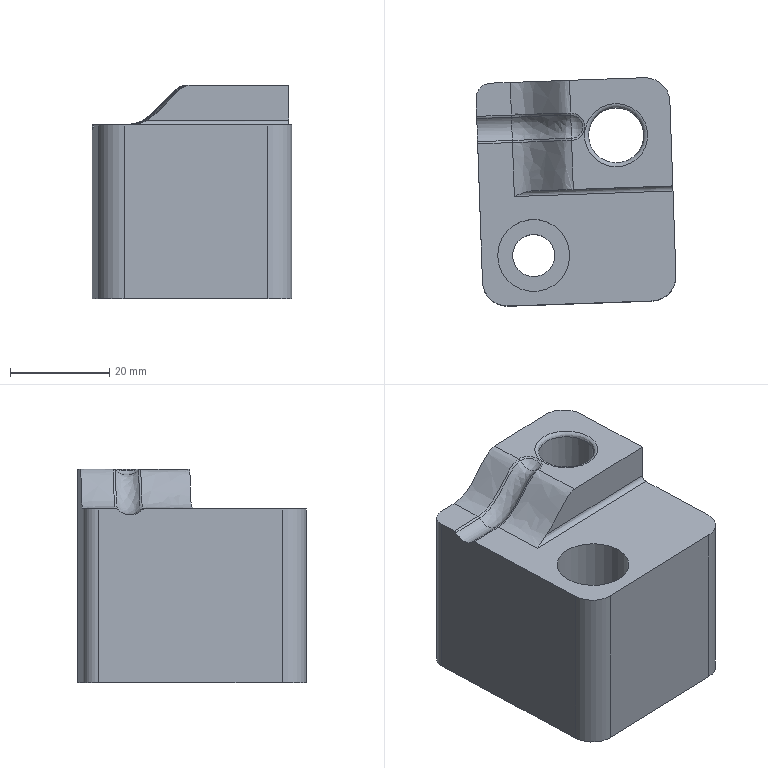Part | NX | features DIE-52 2 | 1 solid | 29 faces | box 40.272 x 45.991 x 43 mm | volume 57298 mm3 | plane 10 | cylinder 10 | spline 8 | torus 1 | commonest cylinder face diameters 10 x3 1.2 x2 2 x1 6 x1 8.5 x1 11.14 x1